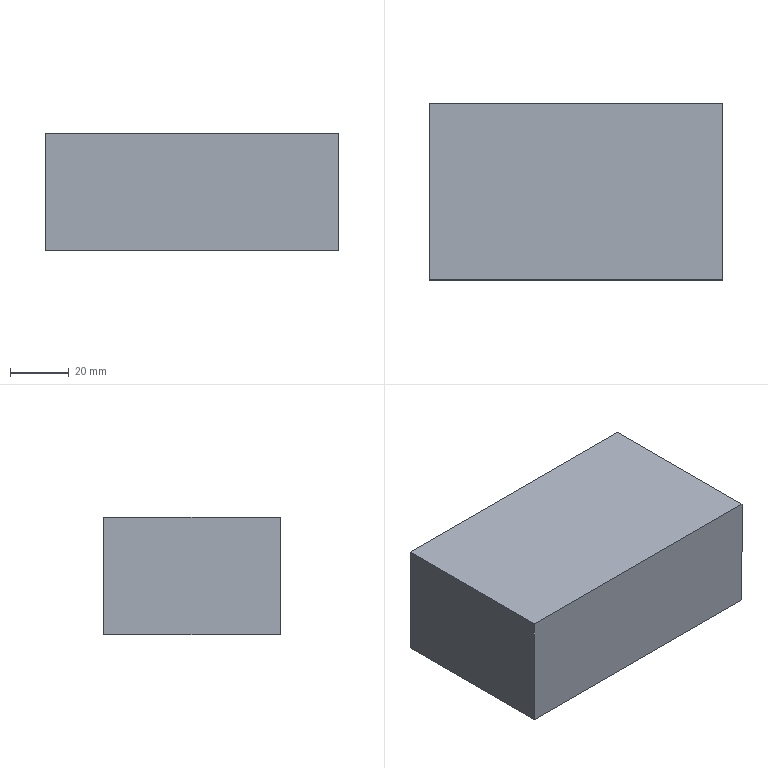Part | STEP file | Part 32 | 1 solid | 6 faces | box 100 x 60 x 40 mm | volume 240000 mm3 | plane 6
STEP:
#1=CARTESIAN_POINT('',(50.,0.,20.));
#2=VERTEX_POINT('',#1);
#3=CARTESIAN_POINT('',(50.,0.,-20.));
#4=VERTEX_POINT('',#3);
#5=CARTESIAN_POINT('',(50.,0.,-20.));
#6=DIRECTION('',(0.,0.,-1.));
#7=VECTOR('',#6,1000.);
#8=LINE('',#5,#7);
#9=EDGE_CURVE('',#2,#4,#8,.T.);
#10=ORIENTED_EDGE('',*,*,#9,.T.);
#11=CARTESIAN_POINT('',(50.,60.,-20.));
#12=VERTEX_POINT('',#11);
#13=CARTESIAN_POINT('',(50.,60.,-20.));
#14=DIRECTION('',(0.,-1.,0.));
#15=VECTOR('',#14,1000.);
#16=LINE('',#13,#15);
#17=EDGE_CURVE('',#12,#4,#16,.T.);
#18=ORIENTED_EDGE('',*,*,#17,.F.);
#19=CARTESIAN_POINT('',(50.,60.,20.));
#20=VERTEX_POINT('',#19);
#21=CARTESIAN_POINT('',(50.,60.,-20.));
#22=DIRECTION('',(0.,0.,-1.));
#23=VECTOR('',#22,1000.);
#24=LINE('',#21,#23);
#25=EDGE_CURVE('',#20,#12,#24,.T.);
#26=ORIENTED_EDGE('',*,*,#25,.F.);
#27=CARTESIAN_POINT('',(50.,60.,20.));
#28=DIRECTION('',(0.,-1.,0.));
#29=VECTOR('',#28,1000.);
#30=LINE('',#27,#29);
#31=EDGE_CURVE('',#20,#2,#30,.T.);
#32=ORIENTED_EDGE('',*,*,#31,.T.);
#33=EDGE_LOOP('',(#10,#18,#26,#32));
#34=FACE_OUTER_BOUND('',#33,.T.);
#35=CARTESIAN_POINT('',(50.,60.,-20.));
#36=DIRECTION('',(-1.,0.,0.));
#37=DIRECTION('',(0.,0.,1.));
#38=AXIS2_PLACEMENT_3D('',#35,#36,#37);
#39=PLANE('',#38);
#40=ADVANCED_FACE('',(#34),#39,.F.);
#41=CARTESIAN_POINT('',(-50.,0.,-20.));
#42=VERTEX_POINT('',#41);
#43=CARTESIAN_POINT('',(-50.,0.,-20.));
#44=DIRECTION('',(-1.,0.,0.));
#45=VECTOR('',#44,1000.);
#46=LINE('',#43,#45);
#47=EDGE_CURVE('',#4,#42,#46,.T.);
#48=ORIENTED_EDGE('',*,*,#47,.T.);
#49=CARTESIAN_POINT('',(-50.,60.,-20.));
#50=VERTEX_POINT('',#49);
#51=CARTESIAN_POINT('',(-50.,60.,-20.));
#52=DIRECTION('',(0.,-1.,0.));
#53=VECTOR('',#52,1000.);
#54=LINE('',#51,#53);
#55=EDGE_CURVE('',#50,#42,#54,.T.);
#56=ORIENTED_EDGE('',*,*,#55,.F.);
#57=CARTESIAN_POINT('',(-50.,60.,-20.));
#58=DIRECTION('',(-1.,0.,0.));
#59=VECTOR('',#58,1000.);
#60=LINE('',#57,#59);
#61=EDGE_CURVE('',#12,#50,#60,.T.);
#62=ORIENTED_EDGE('',*,*,#61,.F.);
#63=ORIENTED_EDGE('',*,*,#17,.T.);
#64=EDGE_LOOP('',(#48,#56,#62,#63));
#65=FACE_OUTER_BOUND('',#64,.T.);
#66=CARTESIAN_POINT('',(-50.,60.,-20.));
#67=DIRECTION('',(0.,0.,1.));
#68=DIRECTION('',(1.,0.,0.));
#69=AXIS2_PLACEMENT_3D('',#66,#67,#68);
#70=PLANE('',#69);
#71=ADVANCED_FACE('',(#65),#70,.F.);
#72=CARTESIAN_POINT('',(-50.,0.,20.));
#73=VERTEX_POINT('',#72);
#74=CARTESIAN_POINT('',(-50.,0.,-20.));
#75=DIRECTION('',(0.,0.,1.));
#76=VECTOR('',#75,1000.);
#77=LINE('',#74,#76);
#78=EDGE_CURVE('',#42,#73,#77,.T.);
#79=ORIENTED_EDGE('',*,*,#78,.T.);
#80=CARTESIAN_POINT('',(-50.,60.,20.));
#81=VERTEX_POINT('',#80);
#82=CARTESIAN_POINT('',(-50.,60.,20.));
#83=DIRECTION('',(0.,-1.,0.));
#84=VECTOR('',#83,1000.);
#85=LINE('',#82,#84);
#86=EDGE_CURVE('',#81,#73,#85,.T.);
#87=ORIENTED_EDGE('',*,*,#86,.F.);
#88=CARTESIAN_POINT('',(-50.,60.,-20.));
#89=DIRECTION('',(0.,0.,1.));
#90=VECTOR('',#89,1000.);
#91=LINE('',#88,#90);
#92=EDGE_CURVE('',#50,#81,#91,.T.);
#93=ORIENTED_EDGE('',*,*,#92,.F.);
#94=ORIENTED_EDGE('',*,*,#55,.T.);
#95=EDGE_LOOP('',(#79,#87,#93,#94));
#96=FACE_OUTER_BOUND('',#95,.T.);
#97=CARTESIAN_POINT('',(-50.,60.,-20.));
#98=DIRECTION('',(1.,0.,0.));
#99=DIRECTION('',(0.,0.,-1.));
#100=AXIS2_PLACEMENT_3D('',#97,#98,#99);
#101=PLANE('',#100);
#102=ADVANCED_FACE('',(#96),#101,.F.);
#103=CARTESIAN_POINT('',(-50.,0.,20.));
#104=DIRECTION('',(1.,0.,0.));
#105=VECTOR('',#104,1000.);
#106=LINE('',#103,#105);
#107=EDGE_CURVE('',#73,#2,#106,.T.);
#108=ORIENTED_EDGE('',*,*,#107,.T.);
#109=ORIENTED_EDGE('',*,*,#31,.F.);
#110=CARTESIAN_POINT('',(-50.,60.,20.));
#111=DIRECTION('',(1.,0.,0.));
#112=VECTOR('',#111,1000.);
#113=LINE('',#110,#112);
#114=EDGE_CURVE('',#81,#20,#113,.T.);
#115=ORIENTED_EDGE('',*,*,#114,.F.);
#116=ORIENTED_EDGE('',*,*,#86,.T.);
#117=EDGE_LOOP('',(#108,#109,#115,#116));
#118=FACE_OUTER_BOUND('',#117,.T.);
#119=CARTESIAN_POINT('',(-50.,60.,20.));
#120=DIRECTION('',(0.,0.,-1.));
#121=DIRECTION('',(-1.,0.,0.));
#122=AXIS2_PLACEMENT_3D('',#119,#120,#121);
#123=PLANE('',#122);
#124=ADVANCED_FACE('',(#118),#123,.F.);
#125=ORIENTED_EDGE('',*,*,#25,.T.);
#126=ORIENTED_EDGE('',*,*,#61,.T.);
#127=ORIENTED_EDGE('',*,*,#92,.T.);
#128=ORIENTED_EDGE('',*,*,#114,.T.);
#129=EDGE_LOOP('',(#125,#126,#127,#128));
#130=FACE_OUTER_BOUND('',#129,.T.);
#131=CARTESIAN_POINT('',(0.,60.,0.));
#132=DIRECTION('',(0.,1.,0.));
#133=DIRECTION('',(0.,0.,1.));
#134=AXIS2_PLACEMENT_3D('',#131,#132,#133);
#135=PLANE('',#134);
#136=ADVANCED_FACE('',(#130),#135,.T.);
#137=ORIENTED_EDGE('',*,*,#9,.F.);
#138=ORIENTED_EDGE('',*,*,#107,.F.);
#139=ORIENTED_EDGE('',*,*,#78,.F.);
#140=ORIENTED_EDGE('',*,*,#47,.F.);
#141=EDGE_LOOP('',(#137,#138,#139,#140));
#142=FACE_OUTER_BOUND('',#141,.T.);
#143=CARTESIAN_POINT('',(0.,0.,0.));
#144=DIRECTION('',(0.,1.,0.));
#145=DIRECTION('',(0.,0.,1.));
#146=AXIS2_PLACEMENT_3D('',#143,#144,#145);
#147=PLANE('',#146);
#148=ADVANCED_FACE('',(#142),#147,.F.);
#149=CLOSED_SHELL('',(#40,#71,#102,#124,#136,#148));
#150=MANIFOLD_SOLID_BREP('',#149);
#151=CARTESIAN_POINT('',(0.,0.,0.));
#152=DIRECTION('',(0.,0.,1.));
#153=DIRECTION('',(1.,0.,0.));
#154=AXIS2_PLACEMENT_3D('',#151,#152,#153);
#155=(LENGTH_UNIT()NAMED_UNIT(*)SI_UNIT(.MILLI.,.METRE.));
#156=UNCERTAINTY_MEASURE_WITH_UNIT(LENGTH_MEASURE(0.00001),#155,'','');
#157=(NAMED_UNIT(*)PLANE_ANGLE_UNIT()SI_UNIT($,.RADIAN.));
#158=(NAMED_UNIT(*)SI_UNIT($,.STERADIAN.)SOLID_ANGLE_UNIT());
#159=(GEOMETRIC_REPRESENTATION_CONTEXT(3)GLOBAL_UNCERTAINTY_ASSIGNED_CONTEXT((#156))GLOBAL_UNIT_ASSIGNED_CONTEXT((#155,#157,#158))REPRESENTATION_CONTEXT('',''));
#160=ADVANCED_BREP_SHAPE_REPRESENTATION('',(#150,#154),#159);